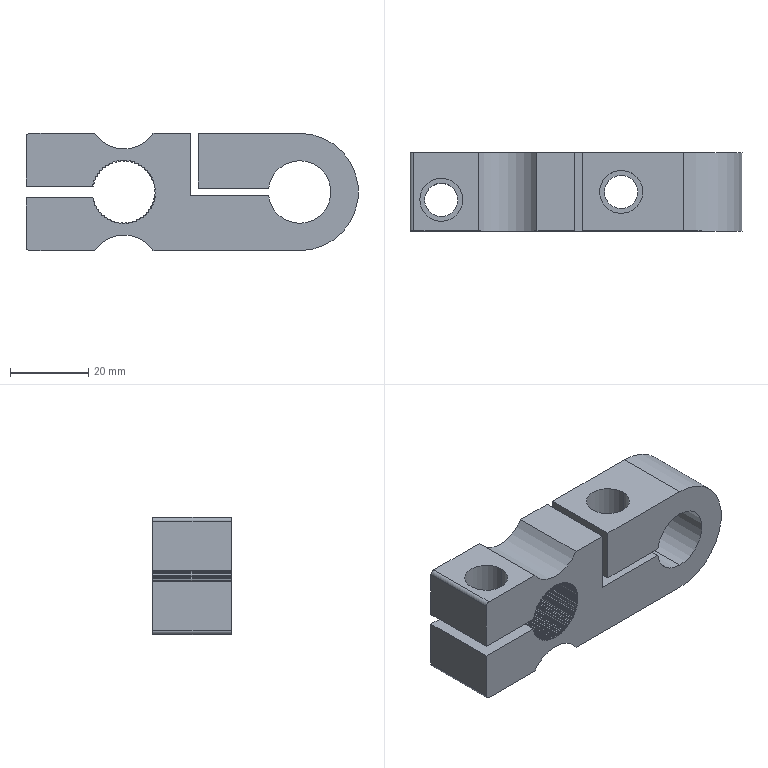Part | SolidWorks | features BaseBody 1 | 1 solid | 276 faces | box 85 x 20 x 30 mm | volume 32752 mm3 | cylinder 168 | plane 108 | commonest cylinder face diameters 0.75 x105 16.285 x46 8.5 x4 11 x4 16 x3 18 x3